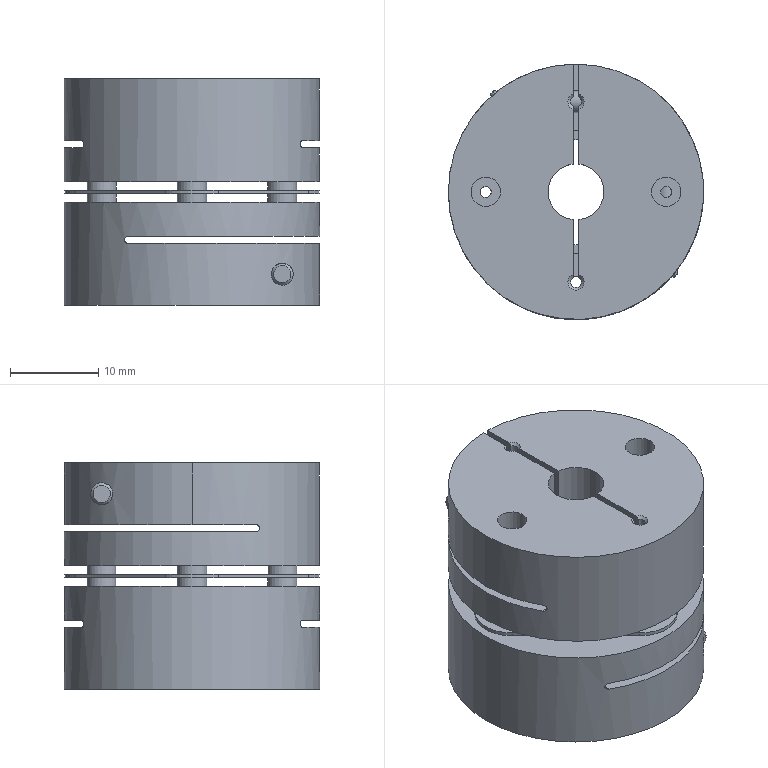Part | STEP file | Diaphragm coupling DEG01-D29-d6.35-e12 | 1 solid | 108 faces | box 29 x 29 x 25.7 mm | volume 11994 mm3 | cylinder 52 | plane 48 | cone 8 | commonest cylinder face diameters 1.25 x12 3.333 x12 2.5 x6 0.83 x4 8.5 x4 14 x3